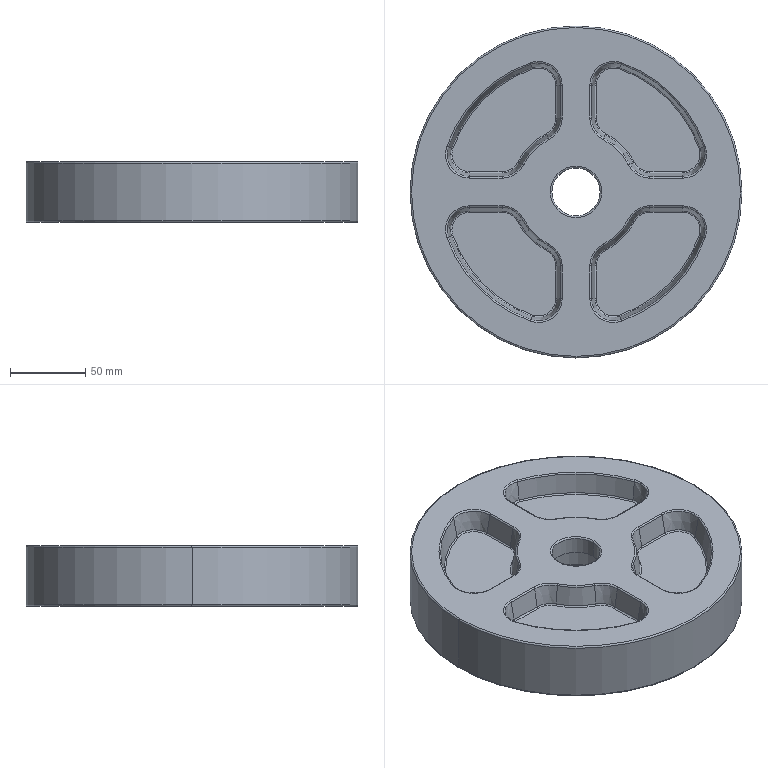Part | SolidWorks | features ICE 7, Fillet 2, CirPattern 1, Extrusion 1, MirrorPattern 1 | 1 solid | 243 faces | box 220 x 220 x 40 mm | volume 1021265 mm3 | torus 112 | cylinder 50 | cone 48 | plane 33 | commonest cylinder face diameters 2 x32 3 x6 52 x4 32 x2 45 x2 55 x2